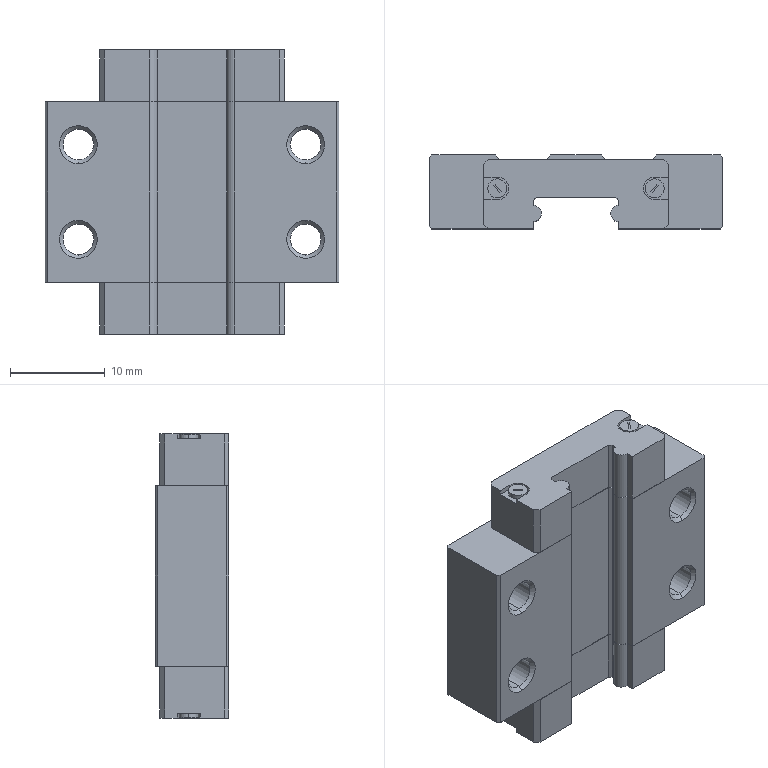Part | STEP file | Linear slider | 1 solid | 183 faces | box 31 x 7.8 x 30 mm | volume 4960 mm3 | plane 130 | cylinder 37 | cone 16 | commonest cylinder face diameters 1.7 x9 2 x8 3.242 x8 1.5 x6 2.4 x6